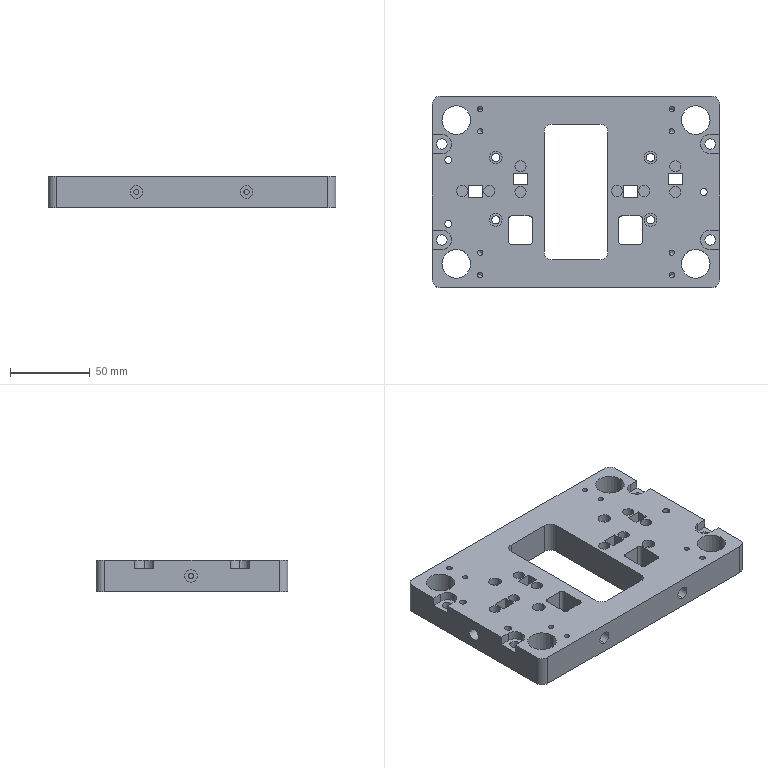Part | STEP file | 03-13 trimming upper blade base plate | 1 solid | 225 faces | box 180 x 120 x 20 mm | volume 311615 mm3 | cylinder 130 | plane 63 | cone 32 | commonest cylinder face diameters 3.3 x40 8 x22 7 x16 4 x8 5.1 x8 6.5 x8